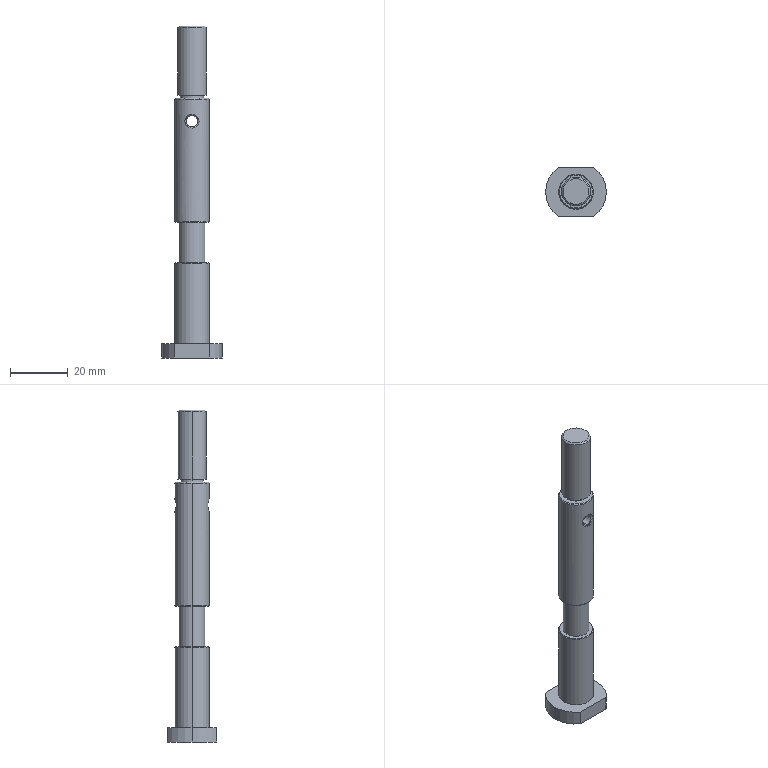Part | STEP file | 101000008214 | 1 solid | 39 faces | box 21 x 17 x 115 mm | volume 12262 mm3 | cylinder 16 | plane 9 | cone 8 | spline 6 | commonest cylinder face diameters 12 x4 21 x4 4 x2 8 x2 9 x2 10 x2